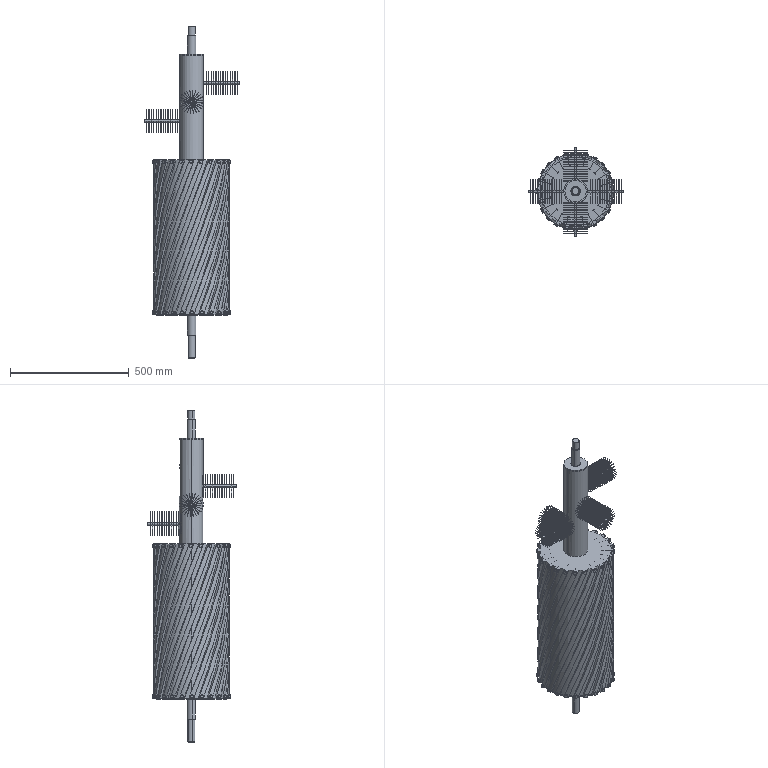Part | SolidWorks | features ReferencePattern 46, LocalCirPattern 2 | 1400 solids | 6620 faces | volume 9398103 mm3 | plane 3195 | cylinder 2863 | cone 394 | spline 168 | commonest cylinder face diameters 1 x2688 8 x99 300 x32 10 x16 40 x8 30 x4